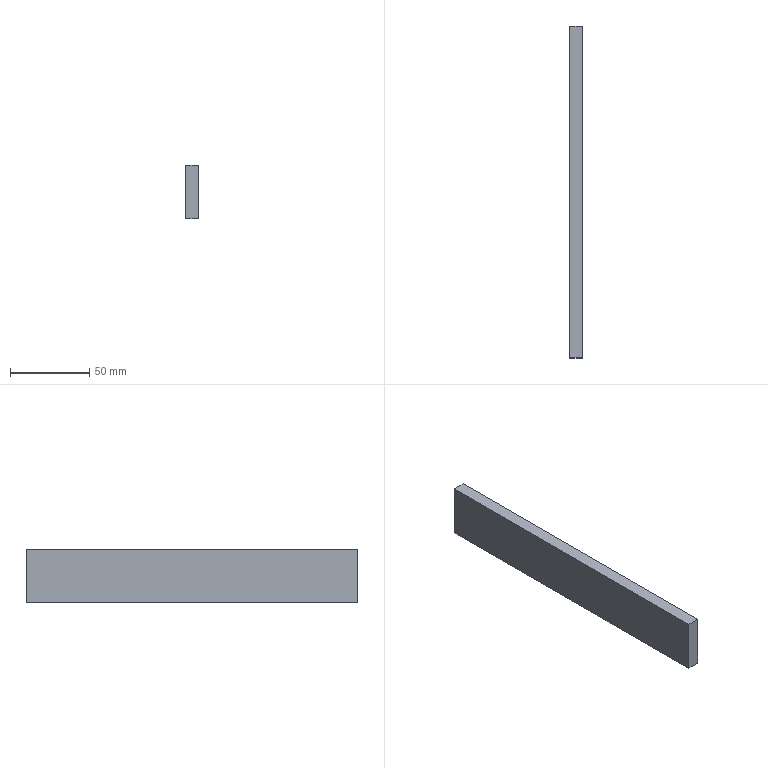Part | SolidWorks | features Extrusion 1 | 1 solid | 6 faces | box 8 x 210 x 34 mm | volume 57120 mm3 | plane 6
STEP:
#1=CARTESIAN_POINT('',(4.,-105.,0.));
#2=VERTEX_POINT('',#1);
#3=CARTESIAN_POINT('',(4.,105.,0.));
#4=VERTEX_POINT('',#3);
#5=CARTESIAN_POINT('',(4.,-105.,0.));
#6=DIRECTION('',(0.,1.,0.));
#7=VECTOR('',#6,1000.);
#8=LINE('',#5,#7);
#9=EDGE_CURVE('',#2,#4,#8,.T.);
#10=ORIENTED_EDGE('',*,*,#9,.T.);
#11=CARTESIAN_POINT('',(4.,105.,34.));
#12=VERTEX_POINT('',#11);
#13=CARTESIAN_POINT('',(4.,105.,34.));
#14=DIRECTION('',(0.,0.,-1.));
#15=VECTOR('',#14,1000.);
#16=LINE('',#13,#15);
#17=EDGE_CURVE('',#12,#4,#16,.T.);
#18=ORIENTED_EDGE('',*,*,#17,.F.);
#19=CARTESIAN_POINT('',(4.,-105.,34.));
#20=VERTEX_POINT('',#19);
#21=CARTESIAN_POINT('',(4.,-105.,34.));
#22=DIRECTION('',(0.,1.,0.));
#23=VECTOR('',#22,1000.);
#24=LINE('',#21,#23);
#25=EDGE_CURVE('',#20,#12,#24,.T.);
#26=ORIENTED_EDGE('',*,*,#25,.F.);
#27=CARTESIAN_POINT('',(4.,-105.,34.));
#28=DIRECTION('',(0.,0.,-1.));
#29=VECTOR('',#28,1000.);
#30=LINE('',#27,#29);
#31=EDGE_CURVE('',#20,#2,#30,.T.);
#32=ORIENTED_EDGE('',*,*,#31,.T.);
#33=EDGE_LOOP('',(#10,#18,#26,#32));
#34=FACE_OUTER_BOUND('',#33,.T.);
#35=CARTESIAN_POINT('',(4.,-105.,34.));
#36=DIRECTION('',(-1.,0.,0.));
#37=DIRECTION('',(0.,0.,1.));
#38=AXIS2_PLACEMENT_3D('',#35,#36,#37);
#39=PLANE('',#38);
#40=ADVANCED_FACE('',(#34),#39,.F.);
#41=CARTESIAN_POINT('',(-4.,105.,0.));
#42=VERTEX_POINT('',#41);
#43=CARTESIAN_POINT('',(-4.,105.,0.));
#44=DIRECTION('',(-1.,0.,0.));
#45=VECTOR('',#44,1000.);
#46=LINE('',#43,#45);
#47=EDGE_CURVE('',#4,#42,#46,.T.);
#48=ORIENTED_EDGE('',*,*,#47,.T.);
#49=CARTESIAN_POINT('',(-4.,105.,34.));
#50=VERTEX_POINT('',#49);
#51=CARTESIAN_POINT('',(-4.,105.,34.));
#52=DIRECTION('',(0.,0.,-1.));
#53=VECTOR('',#52,1000.);
#54=LINE('',#51,#53);
#55=EDGE_CURVE('',#50,#42,#54,.T.);
#56=ORIENTED_EDGE('',*,*,#55,.F.);
#57=CARTESIAN_POINT('',(-4.,105.,34.));
#58=DIRECTION('',(-1.,0.,0.));
#59=VECTOR('',#58,1000.);
#60=LINE('',#57,#59);
#61=EDGE_CURVE('',#12,#50,#60,.T.);
#62=ORIENTED_EDGE('',*,*,#61,.F.);
#63=ORIENTED_EDGE('',*,*,#17,.T.);
#64=EDGE_LOOP('',(#48,#56,#62,#63));
#65=FACE_OUTER_BOUND('',#64,.T.);
#66=CARTESIAN_POINT('',(-4.,105.,34.));
#67=DIRECTION('',(0.,-1.,0.));
#68=DIRECTION('',(0.,0.,-1.));
#69=AXIS2_PLACEMENT_3D('',#66,#67,#68);
#70=PLANE('',#69);
#71=ADVANCED_FACE('',(#65),#70,.F.);
#72=CARTESIAN_POINT('',(-4.,-105.,0.));
#73=VERTEX_POINT('',#72);
#74=CARTESIAN_POINT('',(-4.,-105.,0.));
#75=DIRECTION('',(0.,-1.,0.));
#76=VECTOR('',#75,1000.);
#77=LINE('',#74,#76);
#78=EDGE_CURVE('',#42,#73,#77,.T.);
#79=ORIENTED_EDGE('',*,*,#78,.T.);
#80=CARTESIAN_POINT('',(-4.,-105.,34.));
#81=VERTEX_POINT('',#80);
#82=CARTESIAN_POINT('',(-4.,-105.,34.));
#83=DIRECTION('',(0.,0.,-1.));
#84=VECTOR('',#83,1000.);
#85=LINE('',#82,#84);
#86=EDGE_CURVE('',#81,#73,#85,.T.);
#87=ORIENTED_EDGE('',*,*,#86,.F.);
#88=CARTESIAN_POINT('',(-4.,-105.,34.));
#89=DIRECTION('',(0.,-1.,0.));
#90=VECTOR('',#89,1000.);
#91=LINE('',#88,#90);
#92=EDGE_CURVE('',#50,#81,#91,.T.);
#93=ORIENTED_EDGE('',*,*,#92,.F.);
#94=ORIENTED_EDGE('',*,*,#55,.T.);
#95=EDGE_LOOP('',(#79,#87,#93,#94));
#96=FACE_OUTER_BOUND('',#95,.T.);
#97=CARTESIAN_POINT('',(-4.,-105.,34.));
#98=DIRECTION('',(1.,0.,0.));
#99=DIRECTION('',(0.,0.,-1.));
#100=AXIS2_PLACEMENT_3D('',#97,#98,#99);
#101=PLANE('',#100);
#102=ADVANCED_FACE('',(#96),#101,.F.);
#103=CARTESIAN_POINT('',(-4.,-105.,0.));
#104=DIRECTION('',(1.,0.,0.));
#105=VECTOR('',#104,1000.);
#106=LINE('',#103,#105);
#107=EDGE_CURVE('',#73,#2,#106,.T.);
#108=ORIENTED_EDGE('',*,*,#107,.T.);
#109=ORIENTED_EDGE('',*,*,#31,.F.);
#110=CARTESIAN_POINT('',(-4.,-105.,34.));
#111=DIRECTION('',(1.,0.,0.));
#112=VECTOR('',#111,1000.);
#113=LINE('',#110,#112);
#114=EDGE_CURVE('',#81,#20,#113,.T.);
#115=ORIENTED_EDGE('',*,*,#114,.F.);
#116=ORIENTED_EDGE('',*,*,#86,.T.);
#117=EDGE_LOOP('',(#108,#109,#115,#116));
#118=FACE_OUTER_BOUND('',#117,.T.);
#119=CARTESIAN_POINT('',(-4.,-105.,34.));
#120=DIRECTION('',(0.,1.,0.));
#121=DIRECTION('',(0.,0.,1.));
#122=AXIS2_PLACEMENT_3D('',#119,#120,#121);
#123=PLANE('',#122);
#124=ADVANCED_FACE('',(#118),#123,.F.);
#125=ORIENTED_EDGE('',*,*,#25,.T.);
#126=ORIENTED_EDGE('',*,*,#61,.T.);
#127=ORIENTED_EDGE('',*,*,#92,.T.);
#128=ORIENTED_EDGE('',*,*,#114,.T.);
#129=EDGE_LOOP('',(#125,#126,#127,#128));
#130=FACE_OUTER_BOUND('',#129,.T.);
#131=CARTESIAN_POINT('',(0.,0.,34.));
#132=DIRECTION('',(0.,0.,-1.));
#133=DIRECTION('',(-1.,0.,0.));
#134=AXIS2_PLACEMENT_3D('',#131,#132,#133);
#135=PLANE('',#134);
#136=ADVANCED_FACE('',(#130),#135,.F.);
#137=ORIENTED_EDGE('',*,*,#9,.F.);
#138=ORIENTED_EDGE('',*,*,#107,.F.);
#139=ORIENTED_EDGE('',*,*,#78,.F.);
#140=ORIENTED_EDGE('',*,*,#47,.F.);
#141=EDGE_LOOP('',(#137,#138,#139,#140));
#142=FACE_OUTER_BOUND('',#141,.T.);
#143=CARTESIAN_POINT('',(0.,0.,0.));
#144=DIRECTION('',(0.,0.,-1.));
#145=DIRECTION('',(-1.,0.,0.));
#146=AXIS2_PLACEMENT_3D('',#143,#144,#145);
#147=PLANE('',#146);
#148=ADVANCED_FACE('',(#142),#147,.T.);
#149=CLOSED_SHELL('',(#40,#71,#102,#124,#136,#148));
#150=MANIFOLD_SOLID_BREP('',#149);
#151=CARTESIAN_POINT('',(0.,0.,0.));
#152=DIRECTION('',(0.,0.,1.));
#153=DIRECTION('',(1.,0.,0.));
#154=AXIS2_PLACEMENT_3D('',#151,#152,#153);
#155=(LENGTH_UNIT()NAMED_UNIT(*)SI_UNIT(.MILLI.,.METRE.));
#156=UNCERTAINTY_MEASURE_WITH_UNIT(LENGTH_MEASURE(0.00001),#155,'','');
#157=(NAMED_UNIT(*)PLANE_ANGLE_UNIT()SI_UNIT($,.RADIAN.));
#158=(NAMED_UNIT(*)SI_UNIT($,.STERADIAN.)SOLID_ANGLE_UNIT());
#159=(GEOMETRIC_REPRESENTATION_CONTEXT(3)GLOBAL_UNCERTAINTY_ASSIGNED_CONTEXT((#156))GLOBAL_UNIT_ASSIGNED_CONTEXT((#155,#157,#158))REPRESENTATION_CONTEXT('',''));
#160=ADVANCED_BREP_SHAPE_REPRESENTATION('',(#150,#154),#159);